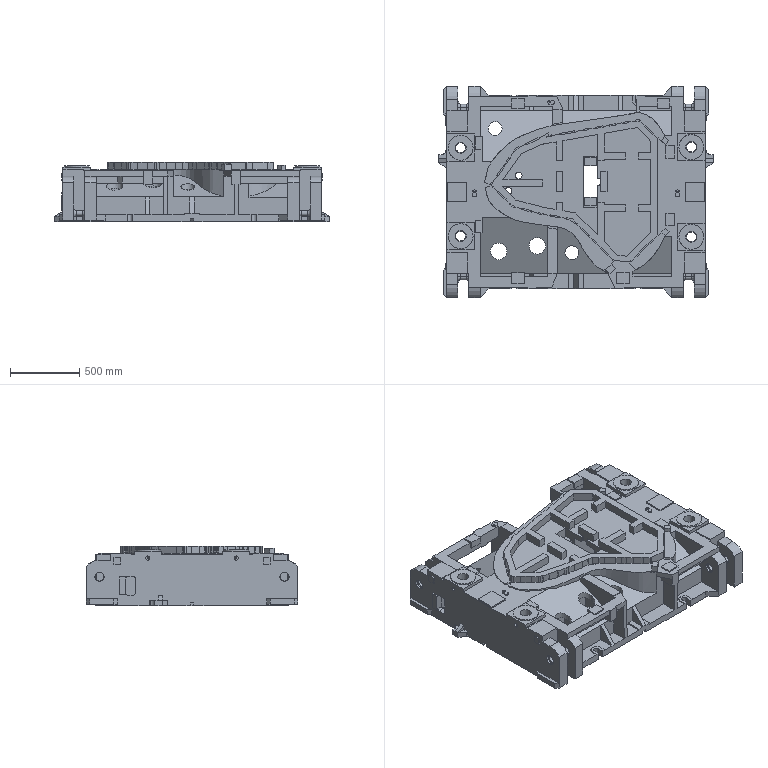Part | NX | features solid 2 | 1 solid | 1260 faces | box 1990 x 1530 x 430 mm | volume 378855644 mm3 | plane 1037 | cylinder 182 | spline 33 | torus 8 | commonest cylinder face diameters 68 x48 40 x44 30 x23 64 x16 10 x10 60 x10